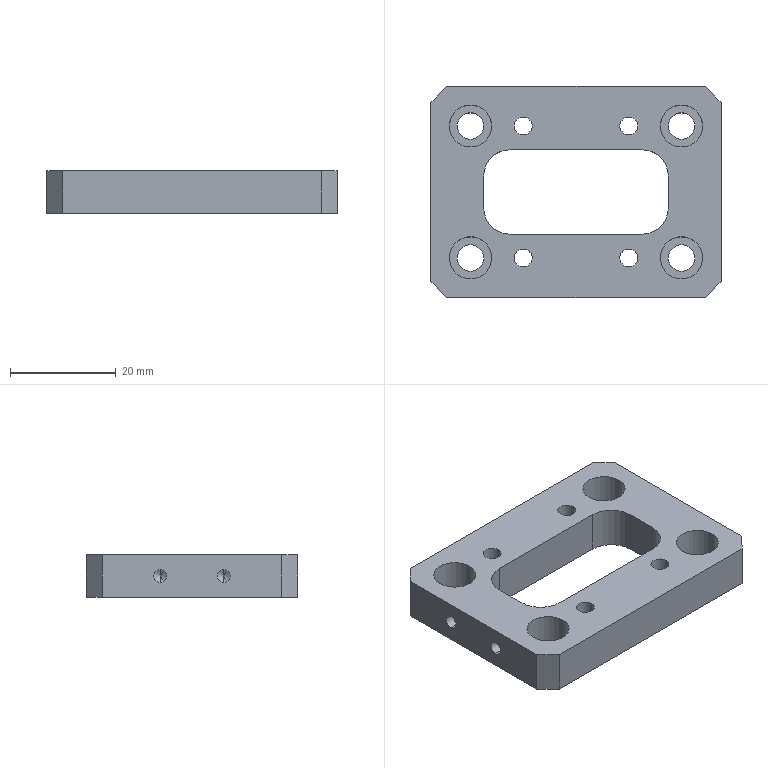Part | SolidWorks | features HoleWzd 4, Chamfer 1, Extrusion 1, Fillet 1, ICE 1 | 1 solid | 74 faces | box 55 x 40 x 8 mm | volume 11071 mm3 | cylinder 44 | plane 22 | cone 8 | commonest cylinder face diameters 2.5 x8 3.4 x8 5 x8 6 x8 8 x8 10 x4